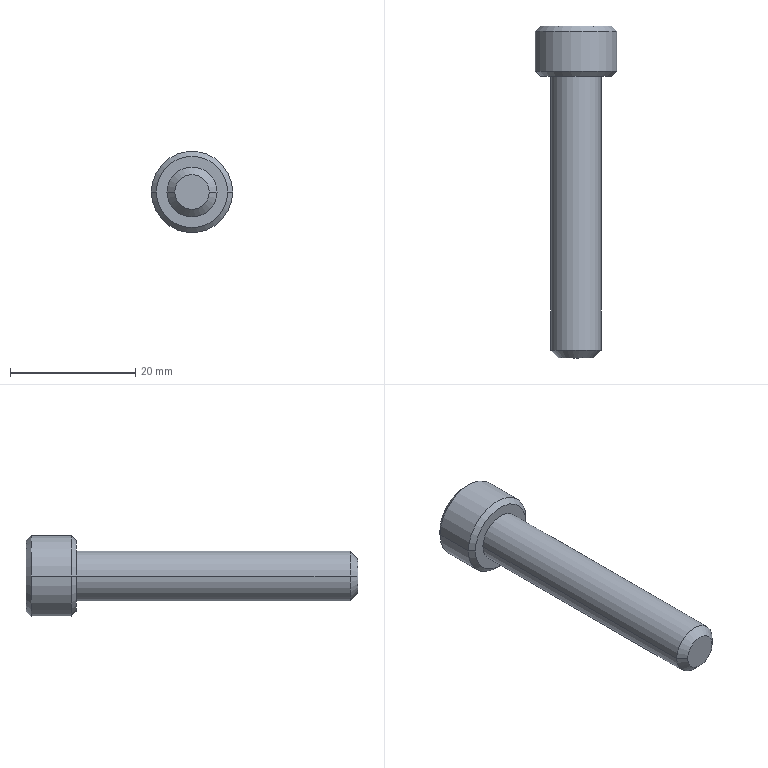Part | STEP file | BB62-M8-45L | 1 solid | 27 faces | box 13 x 53 x 13 mm | volume 3134 mm3 | plane 15 | cone 8 | cylinder 4 | commonest cylinder face diameters 8 x2 13 x2